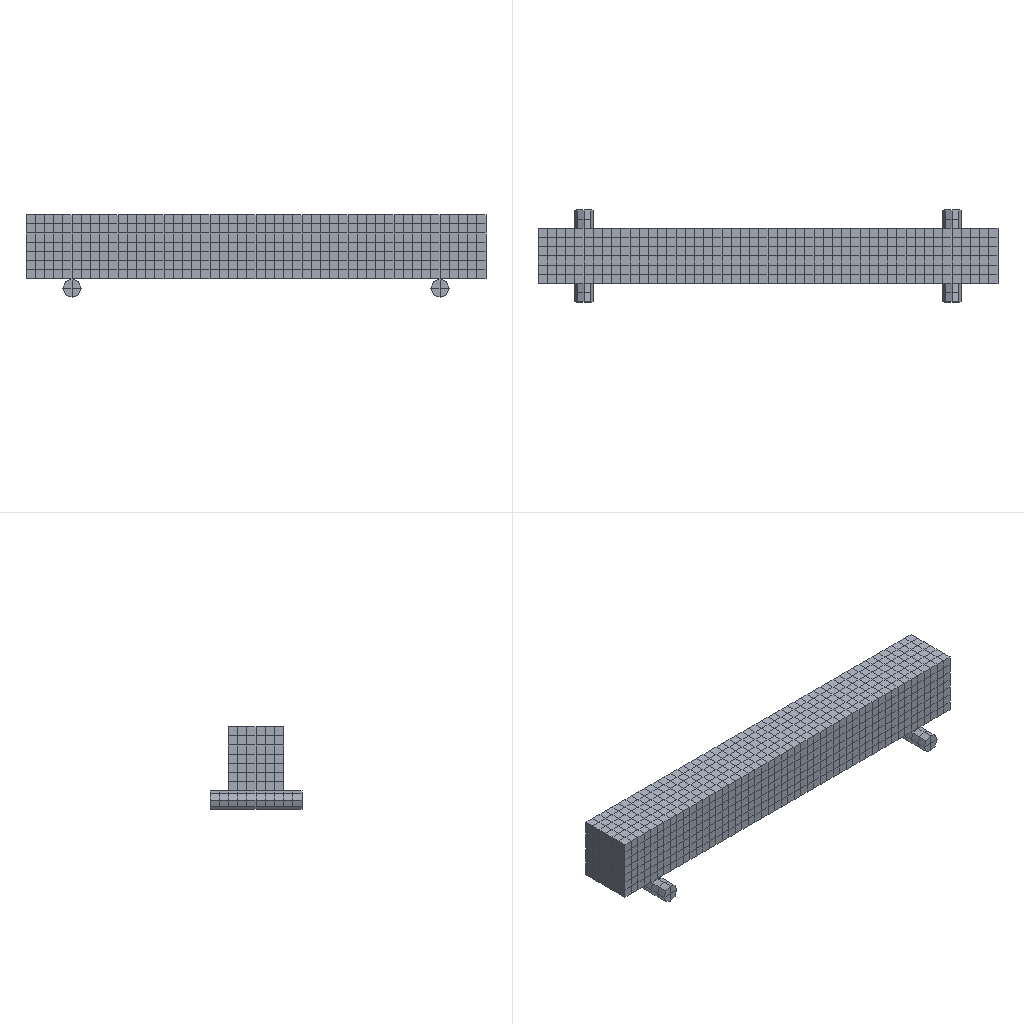Simulation study | abaqus
Set-up summary:
category,name,step,type,value,unit,region
solver,abaqus
solver,version,,,Abaqus/Standard 2020
units,not stated in the deck,,not stated
analysis,deck,,static,static
load_step,Step-1,Step-1,static,nlgeom=True
contact,interactions,,,general=1 pairs=0 ties=0
load_step,requested,,,1
mesh,nodes,,,3454
mesh,elements,,,2380
element_type,T3D2,,truss,200
element_type,C3D8R,,solid,2180
load,load commands in deck,,count,1
bc,support commands in deck,,count,1
material,CON,,in results
material,FIBER,,in results
material,S,,in results
check,setup vs results,,match,"per instance, exact: element labels, types and connectivity; labels of the nodes the elements use; coordinates of those nodes at SINGLE_PRECISION in 2 of 4 instance(s)"
Results summary:
result,step,,completed,increments=66 time=1.0/1.0
result,analysis,,,static
result,last_loadstep,,,1
result,analysis steps,,count,1
result,primary field,,,U
result,reaction total,,FX,-0.5402,model units
result,reaction total,,FY,-0.1668,model units
result,reaction total,,FZ,2085.029,model units